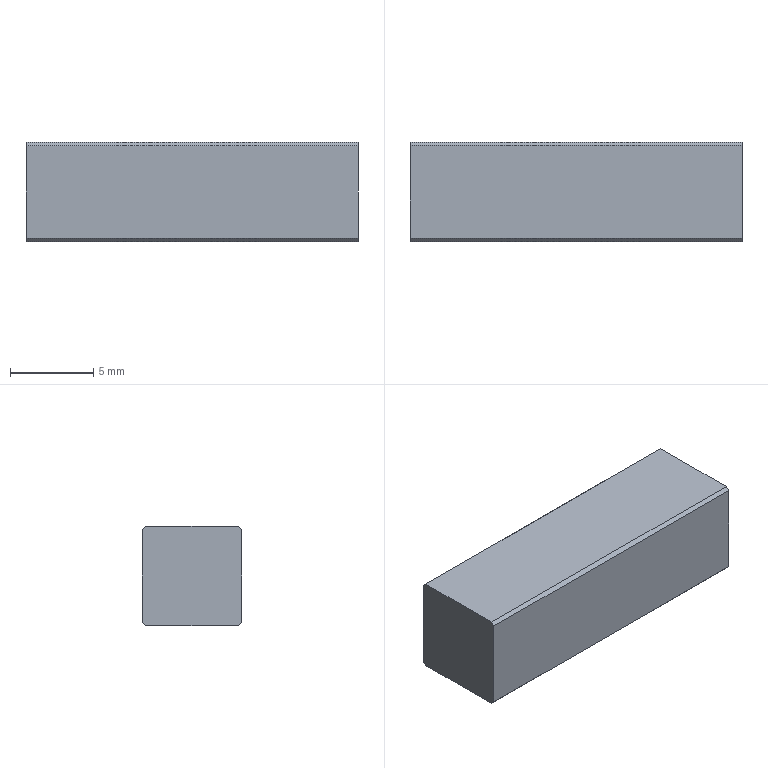Part | STEP file | KEDS6-20 | 1 solid | 10 faces | box 20 x 6 x 6 mm | volume 718.4 mm3 | plane 10
STEP:
#1=CARTESIAN_POINT('',(-10.,6.,-2.8));
#2=VERTEX_POINT('',#1);
#3=CARTESIAN_POINT('',(-10.,6.,2.8));
#4=VERTEX_POINT('',#3);
#5=CARTESIAN_POINT('',(-10.,6.,-3.));
#6=DIRECTION('',(0.,0.,1.));
#7=VECTOR('',#6,1000.);
#8=LINE('',#5,#7);
#9=EDGE_CURVE('',#2,#4,#8,.T.);
#10=ORIENTED_EDGE('',*,*,#9,.F.);
#11=CARTESIAN_POINT('',(-10.,5.8,-3.));
#12=VERTEX_POINT('',#11);
#13=CARTESIAN_POINT('',(-10.,6.,-2.8));
#14=DIRECTION('',(0.,-0.7071,-0.7071));
#15=VECTOR('',#14,1000.);
#16=LINE('',#13,#15);
#17=EDGE_CURVE('',#2,#12,#16,.T.);
#18=ORIENTED_EDGE('',*,*,#17,.T.);
#19=CARTESIAN_POINT('',(-10.,0.2,-3.));
#20=VERTEX_POINT('',#19);
#21=CARTESIAN_POINT('',(-10.,6.,-3.));
#22=DIRECTION('',(0.,-1.,0.));
#23=VECTOR('',#22,1000.);
#24=LINE('',#21,#23);
#25=EDGE_CURVE('',#12,#20,#24,.T.);
#26=ORIENTED_EDGE('',*,*,#25,.T.);
#27=CARTESIAN_POINT('',(-10.,0.,-2.8));
#28=VERTEX_POINT('',#27);
#29=CARTESIAN_POINT('',(-10.,0.2,-3.));
#30=DIRECTION('',(0.,-0.7071,0.7071));
#31=VECTOR('',#30,1000.);
#32=LINE('',#29,#31);
#33=EDGE_CURVE('',#20,#28,#32,.T.);
#34=ORIENTED_EDGE('',*,*,#33,.T.);
#35=CARTESIAN_POINT('',(-10.,0.,2.8));
#36=VERTEX_POINT('',#35);
#37=CARTESIAN_POINT('',(-10.,0.,-3.));
#38=DIRECTION('',(0.,0.,1.));
#39=VECTOR('',#38,1000.);
#40=LINE('',#37,#39);
#41=EDGE_CURVE('',#28,#36,#40,.T.);
#42=ORIENTED_EDGE('',*,*,#41,.T.);
#43=CARTESIAN_POINT('',(-10.,0.2,3.));
#44=VERTEX_POINT('',#43);
#45=CARTESIAN_POINT('',(-10.,0.2,3.));
#46=DIRECTION('',(0.,0.7071,0.7071));
#47=VECTOR('',#46,1000.);
#48=LINE('',#45,#47);
#49=EDGE_CURVE('',#36,#44,#48,.T.);
#50=ORIENTED_EDGE('',*,*,#49,.T.);
#51=CARTESIAN_POINT('',(-10.,5.8,3.));
#52=VERTEX_POINT('',#51);
#53=CARTESIAN_POINT('',(-10.,6.,3.));
#54=DIRECTION('',(0.,-1.,0.));
#55=VECTOR('',#54,1000.);
#56=LINE('',#53,#55);
#57=EDGE_CURVE('',#52,#44,#56,.T.);
#58=ORIENTED_EDGE('',*,*,#57,.F.);
#59=CARTESIAN_POINT('',(-10.,6.,2.8));
#60=DIRECTION('',(0.,0.7071,-0.7071));
#61=VECTOR('',#60,1000.);
#62=LINE('',#59,#61);
#63=EDGE_CURVE('',#52,#4,#62,.T.);
#64=ORIENTED_EDGE('',*,*,#63,.T.);
#65=EDGE_LOOP('',(#10,#18,#26,#34,#42,#50,#58,#64));
#66=FACE_OUTER_BOUND('',#65,.T.);
#67=CARTESIAN_POINT('',(-10.,6.,-3.));
#68=DIRECTION('',(1.,0.,0.));
#69=DIRECTION('',(0.,0.,-1.));
#70=AXIS2_PLACEMENT_3D('',#67,#68,#69);
#71=PLANE('',#70);
#72=ADVANCED_FACE('',(#66),#71,.F.);
#73=ORIENTED_EDGE('',*,*,#57,.T.);
#74=CARTESIAN_POINT('',(10.,0.2,3.));
#75=VERTEX_POINT('',#74);
#76=CARTESIAN_POINT('',(-10.,0.2,3.));
#77=DIRECTION('',(1.,0.,0.));
#78=VECTOR('',#77,1000.);
#79=LINE('',#76,#78);
#80=EDGE_CURVE('',#44,#75,#79,.T.);
#81=ORIENTED_EDGE('',*,*,#80,.T.);
#82=CARTESIAN_POINT('',(10.,5.8,3.));
#83=VERTEX_POINT('',#82);
#84=CARTESIAN_POINT('',(10.,6.,3.));
#85=DIRECTION('',(0.,-1.,0.));
#86=VECTOR('',#85,1000.);
#87=LINE('',#84,#86);
#88=EDGE_CURVE('',#83,#75,#87,.T.);
#89=ORIENTED_EDGE('',*,*,#88,.F.);
#90=CARTESIAN_POINT('',(-10.,5.8,3.));
#91=DIRECTION('',(-1.,0.,0.));
#92=VECTOR('',#91,1000.);
#93=LINE('',#90,#92);
#94=EDGE_CURVE('',#83,#52,#93,.T.);
#95=ORIENTED_EDGE('',*,*,#94,.T.);
#96=EDGE_LOOP('',(#73,#81,#89,#95));
#97=FACE_OUTER_BOUND('',#96,.T.);
#98=CARTESIAN_POINT('',(-10.,6.,3.));
#99=DIRECTION('',(0.,0.,-1.));
#100=DIRECTION('',(-1.,0.,0.));
#101=AXIS2_PLACEMENT_3D('',#98,#99,#100);
#102=PLANE('',#101);
#103=ADVANCED_FACE('',(#97),#102,.F.);
#104=CARTESIAN_POINT('',(10.,5.8,-3.));
#105=VERTEX_POINT('',#104);
#106=CARTESIAN_POINT('',(10.,0.2,-3.));
#107=VERTEX_POINT('',#106);
#108=CARTESIAN_POINT('',(10.,6.,-3.));
#109=DIRECTION('',(0.,-1.,0.));
#110=VECTOR('',#109,1000.);
#111=LINE('',#108,#110);
#112=EDGE_CURVE('',#105,#107,#111,.T.);
#113=ORIENTED_EDGE('',*,*,#112,.F.);
#114=CARTESIAN_POINT('',(10.,6.,-2.8));
#115=VERTEX_POINT('',#114);
#116=CARTESIAN_POINT('',(10.,6.,-2.8));
#117=DIRECTION('',(0.,0.7071,0.7071));
#118=VECTOR('',#117,1000.);
#119=LINE('',#116,#118);
#120=EDGE_CURVE('',#105,#115,#119,.T.);
#121=ORIENTED_EDGE('',*,*,#120,.T.);
#122=CARTESIAN_POINT('',(10.,6.,2.8));
#123=VERTEX_POINT('',#122);
#124=CARTESIAN_POINT('',(10.,6.,-3.));
#125=DIRECTION('',(0.,0.,-1.));
#126=VECTOR('',#125,1000.);
#127=LINE('',#124,#126);
#128=EDGE_CURVE('',#123,#115,#127,.T.);
#129=ORIENTED_EDGE('',*,*,#128,.F.);
#130=CARTESIAN_POINT('',(10.,6.,2.8));
#131=DIRECTION('',(0.,-0.7071,0.7071));
#132=VECTOR('',#131,1000.);
#133=LINE('',#130,#132);
#134=EDGE_CURVE('',#123,#83,#133,.T.);
#135=ORIENTED_EDGE('',*,*,#134,.T.);
#136=ORIENTED_EDGE('',*,*,#88,.T.);
#137=CARTESIAN_POINT('',(10.,0.,2.8));
#138=VERTEX_POINT('',#137);
#139=CARTESIAN_POINT('',(10.,0.2,3.));
#140=DIRECTION('',(0.,-0.7071,-0.7071));
#141=VECTOR('',#140,1000.);
#142=LINE('',#139,#141);
#143=EDGE_CURVE('',#75,#138,#142,.T.);
#144=ORIENTED_EDGE('',*,*,#143,.T.);
#145=CARTESIAN_POINT('',(10.,0.,-2.8));
#146=VERTEX_POINT('',#145);
#147=CARTESIAN_POINT('',(10.,0.,-3.));
#148=DIRECTION('',(0.,0.,-1.));
#149=VECTOR('',#148,1000.);
#150=LINE('',#147,#149);
#151=EDGE_CURVE('',#138,#146,#150,.T.);
#152=ORIENTED_EDGE('',*,*,#151,.T.);
#153=CARTESIAN_POINT('',(10.,0.2,-3.));
#154=DIRECTION('',(0.,0.7071,-0.7071));
#155=VECTOR('',#154,1000.);
#156=LINE('',#153,#155);
#157=EDGE_CURVE('',#146,#107,#156,.T.);
#158=ORIENTED_EDGE('',*,*,#157,.T.);
#159=EDGE_LOOP('',(#113,#121,#129,#135,#136,#144,#152,#158));
#160=FACE_OUTER_BOUND('',#159,.T.);
#161=CARTESIAN_POINT('',(10.,6.,-3.));
#162=DIRECTION('',(-1.,0.,0.));
#163=DIRECTION('',(0.,0.,1.));
#164=AXIS2_PLACEMENT_3D('',#161,#162,#163);
#165=PLANE('',#164);
#166=ADVANCED_FACE('',(#160),#165,.F.);
#167=ORIENTED_EDGE('',*,*,#25,.F.);
#168=CARTESIAN_POINT('',(10.,5.8,-3.));
#169=DIRECTION('',(1.,0.,0.));
#170=VECTOR('',#169,1000.);
#171=LINE('',#168,#170);
#172=EDGE_CURVE('',#12,#105,#171,.T.);
#173=ORIENTED_EDGE('',*,*,#172,.T.);
#174=ORIENTED_EDGE('',*,*,#112,.T.);
#175=CARTESIAN_POINT('',(-10.,0.2,-3.));
#176=DIRECTION('',(-1.,0.,0.));
#177=VECTOR('',#176,1000.);
#178=LINE('',#175,#177);
#179=EDGE_CURVE('',#107,#20,#178,.T.);
#180=ORIENTED_EDGE('',*,*,#179,.T.);
#181=EDGE_LOOP('',(#167,#173,#174,#180));
#182=FACE_OUTER_BOUND('',#181,.T.);
#183=CARTESIAN_POINT('',(-10.,6.,-3.));
#184=DIRECTION('',(0.,0.,1.));
#185=DIRECTION('',(1.,0.,0.));
#186=AXIS2_PLACEMENT_3D('',#183,#184,#185);
#187=PLANE('',#186);
#188=ADVANCED_FACE('',(#182),#187,.F.);
#189=ORIENTED_EDGE('',*,*,#128,.T.);
#190=CARTESIAN_POINT('',(-10.,6.,-2.8));
#191=DIRECTION('',(-1.,0.,0.));
#192=VECTOR('',#191,1000.);
#193=LINE('',#190,#192);
#194=EDGE_CURVE('',#115,#2,#193,.T.);
#195=ORIENTED_EDGE('',*,*,#194,.T.);
#196=ORIENTED_EDGE('',*,*,#9,.T.);
#197=CARTESIAN_POINT('',(10.,6.,2.8));
#198=DIRECTION('',(1.,0.,0.));
#199=VECTOR('',#198,1000.);
#200=LINE('',#197,#199);
#201=EDGE_CURVE('',#4,#123,#200,.T.);
#202=ORIENTED_EDGE('',*,*,#201,.T.);
#203=EDGE_LOOP('',(#189,#195,#196,#202));
#204=FACE_OUTER_BOUND('',#203,.T.);
#205=CARTESIAN_POINT('',(0.,6.,0.));
#206=DIRECTION('',(0.,1.,0.));
#207=DIRECTION('',(0.,0.,1.));
#208=AXIS2_PLACEMENT_3D('',#205,#206,#207);
#209=PLANE('',#208);
#210=ADVANCED_FACE('',(#204),#209,.T.);
#211=ORIENTED_EDGE('',*,*,#41,.F.);
#212=CARTESIAN_POINT('',(0.,0.,-2.8));
#213=DIRECTION('',(1.,0.,0.));
#214=VECTOR('',#213,1000.);
#215=LINE('',#212,#214);
#216=EDGE_CURVE('',#28,#146,#215,.T.);
#217=ORIENTED_EDGE('',*,*,#216,.T.);
#218=ORIENTED_EDGE('',*,*,#151,.F.);
#219=CARTESIAN_POINT('',(0.,0.,2.8));
#220=DIRECTION('',(-1.,0.,0.));
#221=VECTOR('',#220,1000.);
#222=LINE('',#219,#221);
#223=EDGE_CURVE('',#138,#36,#222,.T.);
#224=ORIENTED_EDGE('',*,*,#223,.T.);
#225=EDGE_LOOP('',(#211,#217,#218,#224));
#226=FACE_OUTER_BOUND('',#225,.T.);
#227=CARTESIAN_POINT('',(0.,0.,0.));
#228=DIRECTION('',(0.,1.,0.));
#229=DIRECTION('',(0.,0.,1.));
#230=AXIS2_PLACEMENT_3D('',#227,#228,#229);
#231=PLANE('',#230);
#232=ADVANCED_FACE('',(#226),#231,.F.);
#233=ORIENTED_EDGE('',*,*,#120,.F.);
#234=ORIENTED_EDGE('',*,*,#172,.F.);
#235=ORIENTED_EDGE('',*,*,#17,.F.);
#236=ORIENTED_EDGE('',*,*,#194,.F.);
#237=EDGE_LOOP('',(#233,#234,#235,#236));
#238=FACE_OUTER_BOUND('',#237,.T.);
#239=CARTESIAN_POINT('',(0.,6.,-2.8));
#240=DIRECTION('',(0.,0.7071,-0.7071));
#241=DIRECTION('',(1.,0.,0.));
#242=AXIS2_PLACEMENT_3D('',#239,#240,#241);
#243=PLANE('',#242);
#244=ADVANCED_FACE('',(#238),#243,.T.);
#245=ORIENTED_EDGE('',*,*,#157,.F.);
#246=ORIENTED_EDGE('',*,*,#216,.F.);
#247=ORIENTED_EDGE('',*,*,#33,.F.);
#248=ORIENTED_EDGE('',*,*,#179,.F.);
#249=EDGE_LOOP('',(#245,#246,#247,#248));
#250=FACE_OUTER_BOUND('',#249,.T.);
#251=CARTESIAN_POINT('',(-10.,0.2,-3.));
#252=DIRECTION('',(0.,0.7071,0.7071));
#253=DIRECTION('',(-1.,0.,0.));
#254=AXIS2_PLACEMENT_3D('',#251,#252,#253);
#255=PLANE('',#254);
#256=ADVANCED_FACE('',(#250),#255,.F.);
#257=ORIENTED_EDGE('',*,*,#49,.F.);
#258=ORIENTED_EDGE('',*,*,#223,.F.);
#259=ORIENTED_EDGE('',*,*,#143,.F.);
#260=ORIENTED_EDGE('',*,*,#80,.F.);
#261=EDGE_LOOP('',(#257,#258,#259,#260));
#262=FACE_OUTER_BOUND('',#261,.T.);
#263=CARTESIAN_POINT('',(-10.,0.2,3.));
#264=DIRECTION('',(0.,0.7071,-0.7071));
#265=DIRECTION('',(1.,0.,0.));
#266=AXIS2_PLACEMENT_3D('',#263,#264,#265);
#267=PLANE('',#266);
#268=ADVANCED_FACE('',(#262),#267,.F.);
#269=ORIENTED_EDGE('',*,*,#63,.F.);
#270=ORIENTED_EDGE('',*,*,#94,.F.);
#271=ORIENTED_EDGE('',*,*,#134,.F.);
#272=ORIENTED_EDGE('',*,*,#201,.F.);
#273=EDGE_LOOP('',(#269,#270,#271,#272));
#274=FACE_OUTER_BOUND('',#273,.T.);
#275=CARTESIAN_POINT('',(0.,6.,2.8));
#276=DIRECTION('',(0.,0.7071,0.7071));
#277=DIRECTION('',(-1.,0.,0.));
#278=AXIS2_PLACEMENT_3D('',#275,#276,#277);
#279=PLANE('',#278);
#280=ADVANCED_FACE('',(#274),#279,.T.);
#281=CLOSED_SHELL('',(#72,#103,#166,#188,#210,#232,#244,#256,#268,#280));
#282=MANIFOLD_SOLID_BREP('',#281);
#283=CARTESIAN_POINT('',(0.,0.,0.));
#284=DIRECTION('',(0.,0.,1.));
#285=DIRECTION('',(1.,0.,0.));
#286=AXIS2_PLACEMENT_3D('',#283,#284,#285);
#287=(LENGTH_UNIT()NAMED_UNIT(*)SI_UNIT(.MILLI.,.METRE.));
#288=UNCERTAINTY_MEASURE_WITH_UNIT(LENGTH_MEASURE(0.00001),#287,'','');
#289=(NAMED_UNIT(*)PLANE_ANGLE_UNIT()SI_UNIT($,.RADIAN.));
#290=(NAMED_UNIT(*)SI_UNIT($,.STERADIAN.)SOLID_ANGLE_UNIT());
#291=(GEOMETRIC_REPRESENTATION_CONTEXT(3)GLOBAL_UNCERTAINTY_ASSIGNED_CONTEXT((#288))GLOBAL_UNIT_ASSIGNED_CONTEXT((#287,#289,#290))REPRESENTATION_CONTEXT('',''));
#292=ADVANCED_BREP_SHAPE_REPRESENTATION('',(#282,#286),#291);